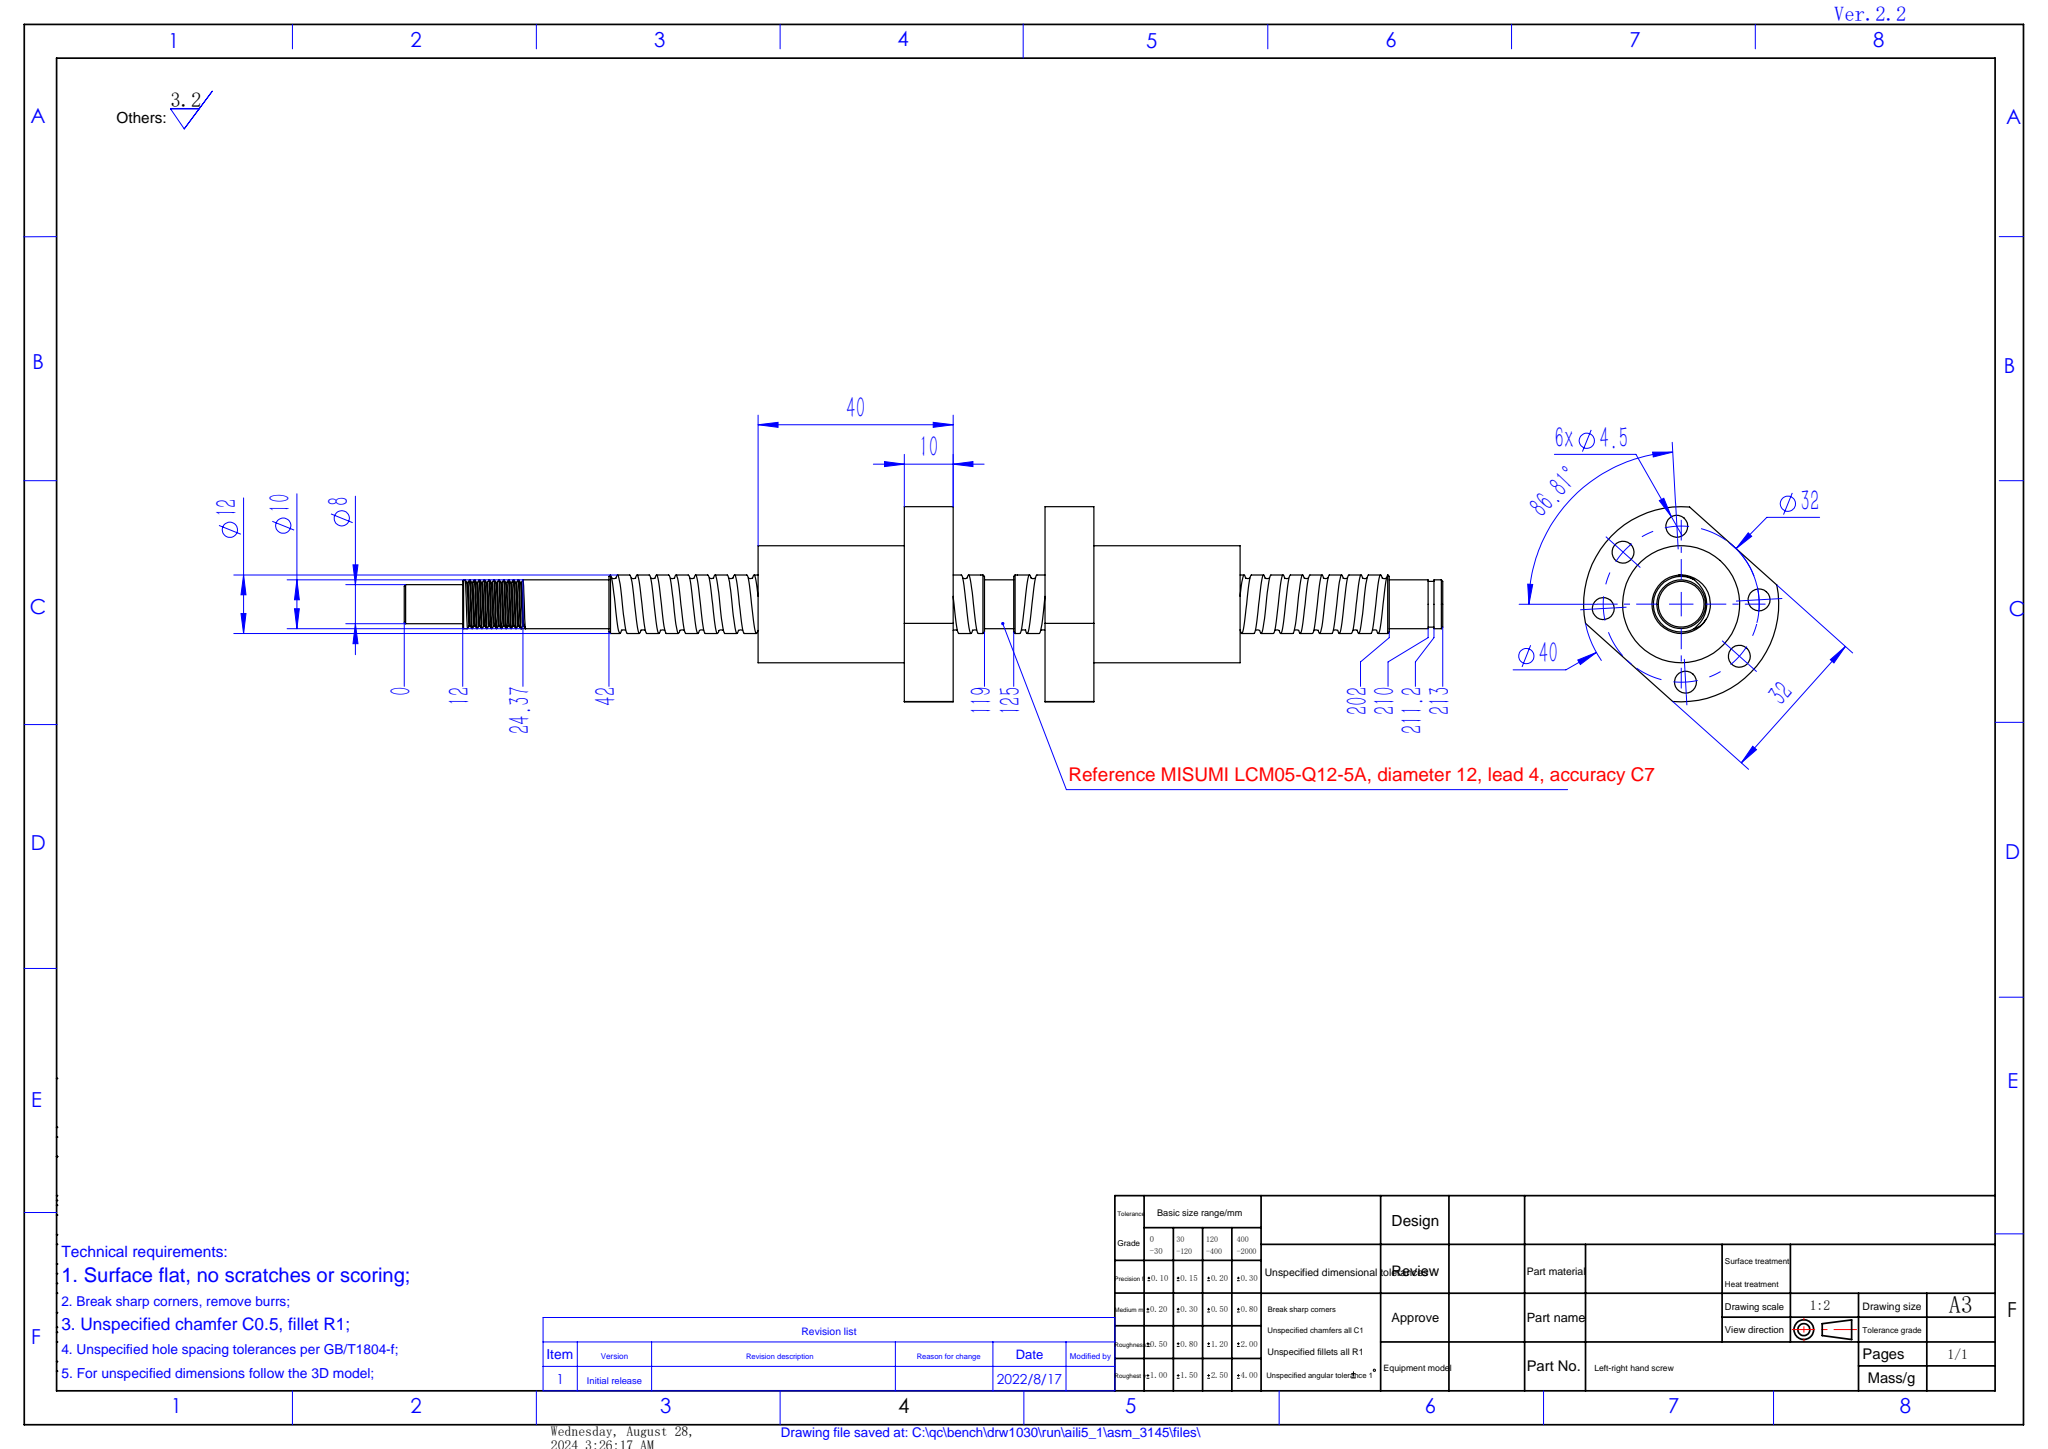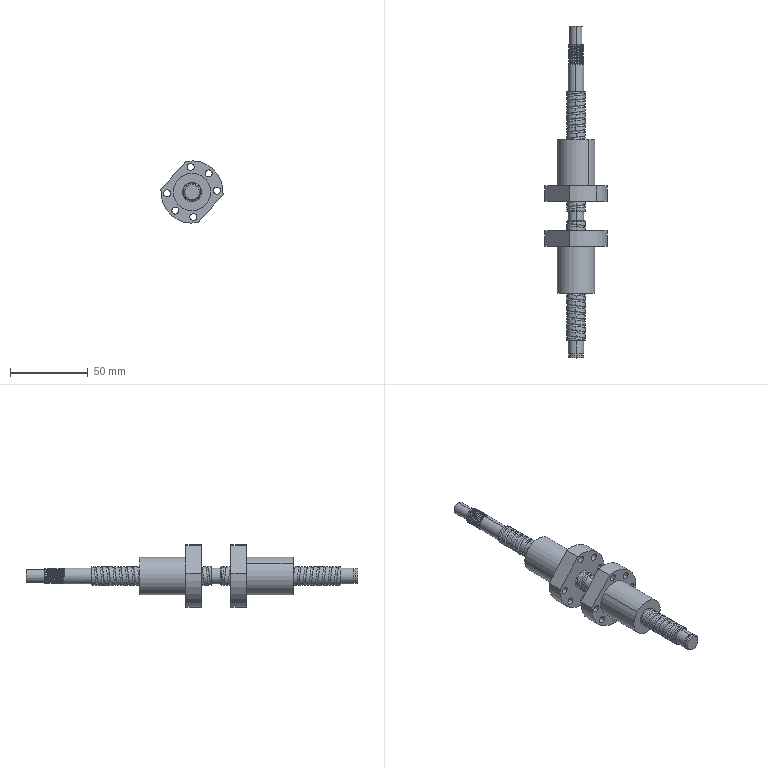Part | SolidWorks | 3 solids | 195 faces | box 40 x 213 x 40 mm | volume 59084 mm3 | cylinder 153 | plane 23 | cone 14 | spline 5 | commonest cylinder face diameters 12 x84 10 x32 4.5 x24 40 x5 24 x4 8 x2